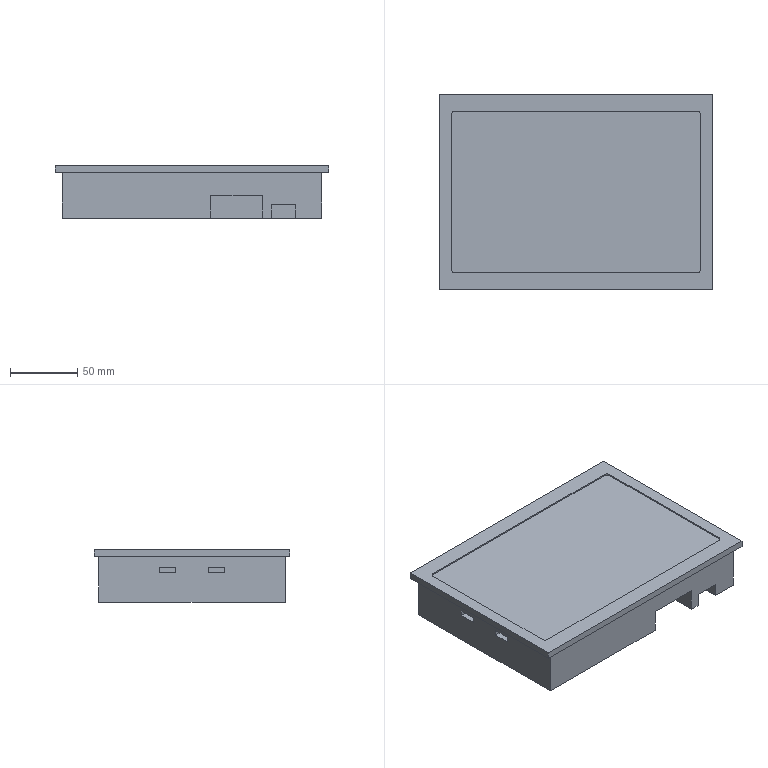Part | STEP file | HMI touch panel SK-070QE.V1.5 | 1 solid | 48 faces | box 203 x 145 x 39 mm | volume 1003292 mm3 | plane 44 | cylinder 4 | commonest cylinder face diameters 6 x4